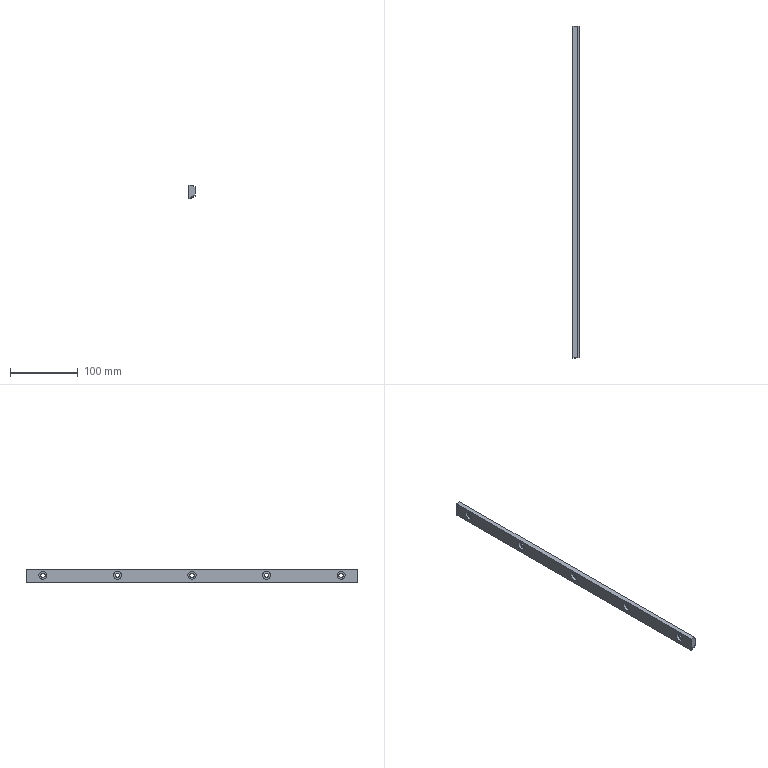Part | STEP file | 1 solid | 43 faces | box 9 x 490 x 20.4 mm | volume 77235 mm3 | cylinder 26 | plane 17 | commonest cylinder face diameters 6.5 x10 12 x10 3 x6